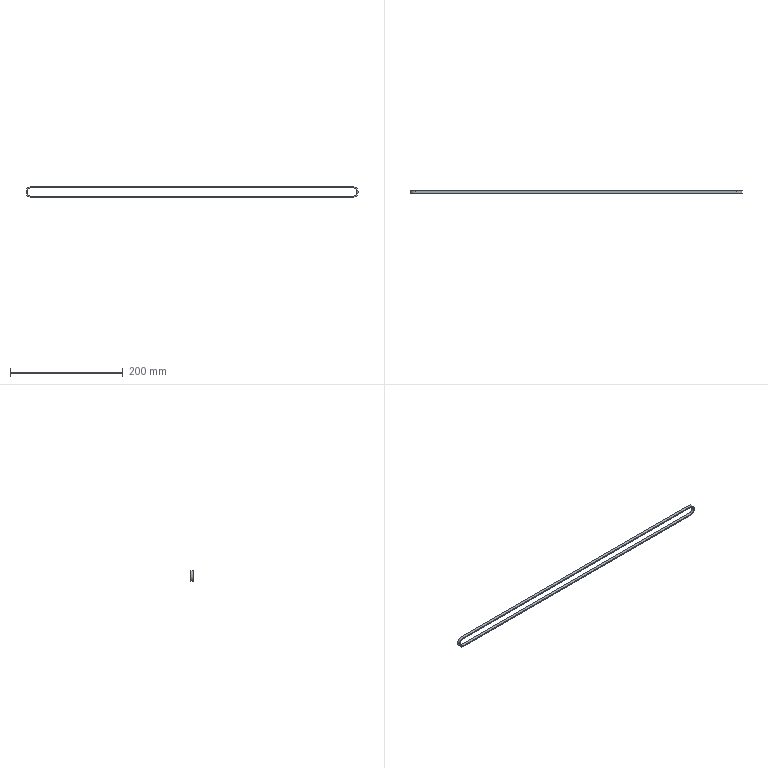Part | SolidWorks | features Extrusion 1 | 1 solid | 10 faces | box 588 x 5 x 19 mm | volume 11914 mm3 | plane 6 | cylinder 4 | commonest cylinder face diameters 15 x2 19 x2
STEP:
#1=CARTESIAN_POINT('',(284.5,5.,9.5));
#2=VERTEX_POINT('',#1);
#3=CARTESIAN_POINT('',(284.5,5.,-9.5));
#4=VERTEX_POINT('',#3);
#5=CARTESIAN_POINT('',(284.5,5.,0.));
#6=DIRECTION('',(0.,1.,0.));
#7=DIRECTION('',(0.,0.,1.));
#8=AXIS2_PLACEMENT_3D('',#5,#6,#7);
#9=CIRCLE('',#8,9.5);
#10=EDGE_CURVE('',#2,#4,#9,.T.);
#11=ORIENTED_EDGE('',*,*,#10,.T.);
#12=CARTESIAN_POINT('',(-284.5,5.,-9.5));
#13=VERTEX_POINT('',#12);
#14=CARTESIAN_POINT('',(284.5,5.,-9.5));
#15=DIRECTION('',(-1.,0.,0.));
#16=VECTOR('',#15,1000.);
#17=LINE('',#14,#16);
#18=EDGE_CURVE('',#4,#13,#17,.T.);
#19=ORIENTED_EDGE('',*,*,#18,.T.);
#20=CARTESIAN_POINT('',(-284.5,5.,9.5));
#21=VERTEX_POINT('',#20);
#22=CARTESIAN_POINT('',(-284.5,5.,0.));
#23=DIRECTION('',(0.,1.,0.));
#24=DIRECTION('',(0.,0.,1.));
#25=AXIS2_PLACEMENT_3D('',#22,#23,#24);
#26=CIRCLE('',#25,9.5);
#27=EDGE_CURVE('',#13,#21,#26,.T.);
#28=ORIENTED_EDGE('',*,*,#27,.T.);
#29=CARTESIAN_POINT('',(284.5,5.,9.5));
#30=DIRECTION('',(1.,0.,0.));
#31=VECTOR('',#30,1000.);
#32=LINE('',#29,#31);
#33=EDGE_CURVE('',#21,#2,#32,.T.);
#34=ORIENTED_EDGE('',*,*,#33,.T.);
#35=EDGE_LOOP('',(#11,#19,#28,#34));
#36=FACE_OUTER_BOUND('',#35,.T.);
#37=CARTESIAN_POINT('',(284.5,5.,-7.5));
#38=VERTEX_POINT('',#37);
#39=CARTESIAN_POINT('',(-284.5,5.,-7.5));
#40=VERTEX_POINT('',#39);
#41=CARTESIAN_POINT('',(284.5,5.,-7.5));
#42=DIRECTION('',(-1.,0.,0.));
#43=VECTOR('',#42,1000.);
#44=LINE('',#41,#43);
#45=EDGE_CURVE('',#38,#40,#44,.T.);
#46=ORIENTED_EDGE('',*,*,#45,.F.);
#47=CARTESIAN_POINT('',(284.5,5.,7.5));
#48=VERTEX_POINT('',#47);
#49=CARTESIAN_POINT('',(284.5,5.,0.));
#50=DIRECTION('',(0.,1.,0.));
#51=DIRECTION('',(0.,0.,1.));
#52=AXIS2_PLACEMENT_3D('',#49,#50,#51);
#53=CIRCLE('',#52,7.5);
#54=EDGE_CURVE('',#48,#38,#53,.T.);
#55=ORIENTED_EDGE('',*,*,#54,.F.);
#56=CARTESIAN_POINT('',(-284.5,5.,7.5));
#57=VERTEX_POINT('',#56);
#58=CARTESIAN_POINT('',(284.5,5.,7.5));
#59=DIRECTION('',(1.,0.,0.));
#60=VECTOR('',#59,1000.);
#61=LINE('',#58,#60);
#62=EDGE_CURVE('',#57,#48,#61,.T.);
#63=ORIENTED_EDGE('',*,*,#62,.F.);
#64=CARTESIAN_POINT('',(-284.5,5.,0.));
#65=DIRECTION('',(0.,1.,0.));
#66=DIRECTION('',(0.,0.,1.));
#67=AXIS2_PLACEMENT_3D('',#64,#65,#66);
#68=CIRCLE('',#67,7.5);
#69=EDGE_CURVE('',#40,#57,#68,.T.);
#70=ORIENTED_EDGE('',*,*,#69,.F.);
#71=EDGE_LOOP('',(#46,#55,#63,#70));
#72=FACE_BOUND('',#71,.T.);
#73=CARTESIAN_POINT('',(284.5,5.,0.));
#74=DIRECTION('',(0.,1.,0.));
#75=DIRECTION('',(0.,0.,1.));
#76=AXIS2_PLACEMENT_3D('',#73,#74,#75);
#77=PLANE('',#76);
#78=ADVANCED_FACE('',(#36,#72),#77,.T.);
#79=CARTESIAN_POINT('',(284.5,0.,9.5));
#80=VERTEX_POINT('',#79);
#81=CARTESIAN_POINT('',(284.5,0.,-9.5));
#82=VERTEX_POINT('',#81);
#83=CARTESIAN_POINT('',(284.5,0.,0.));
#84=DIRECTION('',(0.,1.,0.));
#85=DIRECTION('',(0.,0.,1.));
#86=AXIS2_PLACEMENT_3D('',#83,#84,#85);
#87=CIRCLE('',#86,9.5);
#88=EDGE_CURVE('',#80,#82,#87,.T.);
#89=ORIENTED_EDGE('',*,*,#88,.F.);
#90=CARTESIAN_POINT('',(-284.5,0.,9.5));
#91=VERTEX_POINT('',#90);
#92=CARTESIAN_POINT('',(284.5,0.,9.5));
#93=DIRECTION('',(1.,0.,0.));
#94=VECTOR('',#93,1000.);
#95=LINE('',#92,#94);
#96=EDGE_CURVE('',#91,#80,#95,.T.);
#97=ORIENTED_EDGE('',*,*,#96,.F.);
#98=CARTESIAN_POINT('',(-284.5,0.,-9.5));
#99=VERTEX_POINT('',#98);
#100=CARTESIAN_POINT('',(-284.5,0.,0.));
#101=DIRECTION('',(0.,1.,0.));
#102=DIRECTION('',(0.,0.,1.));
#103=AXIS2_PLACEMENT_3D('',#100,#101,#102);
#104=CIRCLE('',#103,9.5);
#105=EDGE_CURVE('',#99,#91,#104,.T.);
#106=ORIENTED_EDGE('',*,*,#105,.F.);
#107=CARTESIAN_POINT('',(284.5,0.,-9.5));
#108=DIRECTION('',(-1.,0.,0.));
#109=VECTOR('',#108,1000.);
#110=LINE('',#107,#109);
#111=EDGE_CURVE('',#82,#99,#110,.T.);
#112=ORIENTED_EDGE('',*,*,#111,.F.);
#113=EDGE_LOOP('',(#89,#97,#106,#112));
#114=FACE_OUTER_BOUND('',#113,.T.);
#115=CARTESIAN_POINT('',(284.5,0.,7.5));
#116=VERTEX_POINT('',#115);
#117=CARTESIAN_POINT('',(284.5,0.,-7.5));
#118=VERTEX_POINT('',#117);
#119=CARTESIAN_POINT('',(284.5,0.,0.));
#120=DIRECTION('',(0.,1.,0.));
#121=DIRECTION('',(0.,0.,1.));
#122=AXIS2_PLACEMENT_3D('',#119,#120,#121);
#123=CIRCLE('',#122,7.5);
#124=EDGE_CURVE('',#116,#118,#123,.T.);
#125=ORIENTED_EDGE('',*,*,#124,.T.);
#126=CARTESIAN_POINT('',(-284.5,0.,-7.5));
#127=VERTEX_POINT('',#126);
#128=CARTESIAN_POINT('',(284.5,0.,-7.5));
#129=DIRECTION('',(-1.,0.,0.));
#130=VECTOR('',#129,1000.);
#131=LINE('',#128,#130);
#132=EDGE_CURVE('',#118,#127,#131,.T.);
#133=ORIENTED_EDGE('',*,*,#132,.T.);
#134=CARTESIAN_POINT('',(-284.5,0.,7.5));
#135=VERTEX_POINT('',#134);
#136=CARTESIAN_POINT('',(-284.5,0.,0.));
#137=DIRECTION('',(0.,1.,0.));
#138=DIRECTION('',(0.,0.,1.));
#139=AXIS2_PLACEMENT_3D('',#136,#137,#138);
#140=CIRCLE('',#139,7.5);
#141=EDGE_CURVE('',#127,#135,#140,.T.);
#142=ORIENTED_EDGE('',*,*,#141,.T.);
#143=CARTESIAN_POINT('',(284.5,0.,7.5));
#144=DIRECTION('',(1.,0.,0.));
#145=VECTOR('',#144,1000.);
#146=LINE('',#143,#145);
#147=EDGE_CURVE('',#135,#116,#146,.T.);
#148=ORIENTED_EDGE('',*,*,#147,.T.);
#149=EDGE_LOOP('',(#125,#133,#142,#148));
#150=FACE_BOUND('',#149,.T.);
#151=CARTESIAN_POINT('',(284.5,0.,0.));
#152=DIRECTION('',(0.,1.,0.));
#153=DIRECTION('',(0.,0.,1.));
#154=AXIS2_PLACEMENT_3D('',#151,#152,#153);
#155=PLANE('',#154);
#156=ADVANCED_FACE('',(#114,#150),#155,.F.);
#157=ORIENTED_EDGE('',*,*,#88,.T.);
#158=CARTESIAN_POINT('',(284.5,5.,-9.5));
#159=DIRECTION('',(0.,-1.,0.));
#160=VECTOR('',#159,1000.);
#161=LINE('',#158,#160);
#162=EDGE_CURVE('',#4,#82,#161,.T.);
#163=ORIENTED_EDGE('',*,*,#162,.F.);
#164=ORIENTED_EDGE('',*,*,#10,.F.);
#165=CARTESIAN_POINT('',(284.5,5.,9.5));
#166=DIRECTION('',(0.,-1.,0.));
#167=VECTOR('',#166,1000.);
#168=LINE('',#165,#167);
#169=EDGE_CURVE('',#2,#80,#168,.T.);
#170=ORIENTED_EDGE('',*,*,#169,.T.);
#171=EDGE_LOOP('',(#157,#163,#164,#170));
#172=FACE_OUTER_BOUND('',#171,.T.);
#173=CARTESIAN_POINT('',(284.5,5.,0.));
#174=DIRECTION('',(0.,-1.,0.));
#175=DIRECTION('',(0.,0.,-1.));
#176=AXIS2_PLACEMENT_3D('',#173,#174,#175);
#177=CYLINDRICAL_SURFACE('',#176,9.5);
#178=ADVANCED_FACE('',(#172),#177,.T.);
#179=ORIENTED_EDGE('',*,*,#111,.T.);
#180=CARTESIAN_POINT('',(-284.5,5.,-9.5));
#181=DIRECTION('',(0.,-1.,0.));
#182=VECTOR('',#181,1000.);
#183=LINE('',#180,#182);
#184=EDGE_CURVE('',#13,#99,#183,.T.);
#185=ORIENTED_EDGE('',*,*,#184,.F.);
#186=ORIENTED_EDGE('',*,*,#18,.F.);
#187=ORIENTED_EDGE('',*,*,#162,.T.);
#188=EDGE_LOOP('',(#179,#185,#186,#187));
#189=FACE_OUTER_BOUND('',#188,.T.);
#190=CARTESIAN_POINT('',(284.5,5.,-9.5));
#191=DIRECTION('',(0.,0.,1.));
#192=DIRECTION('',(1.,0.,0.));
#193=AXIS2_PLACEMENT_3D('',#190,#191,#192);
#194=PLANE('',#193);
#195=ADVANCED_FACE('',(#189),#194,.F.);
#196=ORIENTED_EDGE('',*,*,#105,.T.);
#197=CARTESIAN_POINT('',(-284.5,5.,9.5));
#198=DIRECTION('',(0.,-1.,0.));
#199=VECTOR('',#198,1000.);
#200=LINE('',#197,#199);
#201=EDGE_CURVE('',#21,#91,#200,.T.);
#202=ORIENTED_EDGE('',*,*,#201,.F.);
#203=ORIENTED_EDGE('',*,*,#27,.F.);
#204=ORIENTED_EDGE('',*,*,#184,.T.);
#205=EDGE_LOOP('',(#196,#202,#203,#204));
#206=FACE_OUTER_BOUND('',#205,.T.);
#207=CARTESIAN_POINT('',(-284.5,5.,0.));
#208=DIRECTION('',(0.,-1.,0.));
#209=DIRECTION('',(0.,0.,-1.));
#210=AXIS2_PLACEMENT_3D('',#207,#208,#209);
#211=CYLINDRICAL_SURFACE('',#210,9.5);
#212=ADVANCED_FACE('',(#206),#211,.T.);
#213=ORIENTED_EDGE('',*,*,#96,.T.);
#214=ORIENTED_EDGE('',*,*,#169,.F.);
#215=ORIENTED_EDGE('',*,*,#33,.F.);
#216=ORIENTED_EDGE('',*,*,#201,.T.);
#217=EDGE_LOOP('',(#213,#214,#215,#216));
#218=FACE_OUTER_BOUND('',#217,.T.);
#219=CARTESIAN_POINT('',(284.5,5.,9.5));
#220=DIRECTION('',(0.,0.,-1.));
#221=DIRECTION('',(-1.,0.,0.));
#222=AXIS2_PLACEMENT_3D('',#219,#220,#221);
#223=PLANE('',#222);
#224=ADVANCED_FACE('',(#218),#223,.F.);
#225=ORIENTED_EDGE('',*,*,#124,.F.);
#226=CARTESIAN_POINT('',(284.5,5.,7.5));
#227=DIRECTION('',(0.,-1.,0.));
#228=VECTOR('',#227,1000.);
#229=LINE('',#226,#228);
#230=EDGE_CURVE('',#48,#116,#229,.T.);
#231=ORIENTED_EDGE('',*,*,#230,.F.);
#232=ORIENTED_EDGE('',*,*,#54,.T.);
#233=CARTESIAN_POINT('',(284.5,5.,-7.5));
#234=DIRECTION('',(0.,-1.,0.));
#235=VECTOR('',#234,1000.);
#236=LINE('',#233,#235);
#237=EDGE_CURVE('',#38,#118,#236,.T.);
#238=ORIENTED_EDGE('',*,*,#237,.T.);
#239=EDGE_LOOP('',(#225,#231,#232,#238));
#240=FACE_OUTER_BOUND('',#239,.T.);
#241=CARTESIAN_POINT('',(284.5,5.,0.));
#242=DIRECTION('',(0.,-1.,0.));
#243=DIRECTION('',(0.,0.,-1.));
#244=AXIS2_PLACEMENT_3D('',#241,#242,#243);
#245=CYLINDRICAL_SURFACE('',#244,7.5);
#246=ADVANCED_FACE('',(#240),#245,.F.);
#247=ORIENTED_EDGE('',*,*,#132,.F.);
#248=ORIENTED_EDGE('',*,*,#237,.F.);
#249=ORIENTED_EDGE('',*,*,#45,.T.);
#250=CARTESIAN_POINT('',(-284.5,5.,-7.5));
#251=DIRECTION('',(0.,-1.,0.));
#252=VECTOR('',#251,1000.);
#253=LINE('',#250,#252);
#254=EDGE_CURVE('',#40,#127,#253,.T.);
#255=ORIENTED_EDGE('',*,*,#254,.T.);
#256=EDGE_LOOP('',(#247,#248,#249,#255));
#257=FACE_OUTER_BOUND('',#256,.T.);
#258=CARTESIAN_POINT('',(284.5,5.,-7.5));
#259=DIRECTION('',(0.,0.,1.));
#260=DIRECTION('',(1.,0.,0.));
#261=AXIS2_PLACEMENT_3D('',#258,#259,#260);
#262=PLANE('',#261);
#263=ADVANCED_FACE('',(#257),#262,.T.);
#264=ORIENTED_EDGE('',*,*,#141,.F.);
#265=ORIENTED_EDGE('',*,*,#254,.F.);
#266=ORIENTED_EDGE('',*,*,#69,.T.);
#267=CARTESIAN_POINT('',(-284.5,5.,7.5));
#268=DIRECTION('',(0.,-1.,0.));
#269=VECTOR('',#268,1000.);
#270=LINE('',#267,#269);
#271=EDGE_CURVE('',#57,#135,#270,.T.);
#272=ORIENTED_EDGE('',*,*,#271,.T.);
#273=EDGE_LOOP('',(#264,#265,#266,#272));
#274=FACE_OUTER_BOUND('',#273,.T.);
#275=CARTESIAN_POINT('',(-284.5,5.,0.));
#276=DIRECTION('',(0.,-1.,0.));
#277=DIRECTION('',(0.,0.,-1.));
#278=AXIS2_PLACEMENT_3D('',#275,#276,#277);
#279=CYLINDRICAL_SURFACE('',#278,7.5);
#280=ADVANCED_FACE('',(#274),#279,.F.);
#281=ORIENTED_EDGE('',*,*,#147,.F.);
#282=ORIENTED_EDGE('',*,*,#271,.F.);
#283=ORIENTED_EDGE('',*,*,#62,.T.);
#284=ORIENTED_EDGE('',*,*,#230,.T.);
#285=EDGE_LOOP('',(#281,#282,#283,#284));
#286=FACE_OUTER_BOUND('',#285,.T.);
#287=CARTESIAN_POINT('',(284.5,5.,7.5));
#288=DIRECTION('',(0.,0.,-1.));
#289=DIRECTION('',(-1.,0.,0.));
#290=AXIS2_PLACEMENT_3D('',#287,#288,#289);
#291=PLANE('',#290);
#292=ADVANCED_FACE('',(#286),#291,.T.);
#293=CLOSED_SHELL('',(#78,#156,#178,#195,#212,#224,#246,#263,#280,#292));
#294=MANIFOLD_SOLID_BREP('',#293);
#295=CARTESIAN_POINT('',(0.,0.,0.));
#296=DIRECTION('',(0.,0.,1.));
#297=DIRECTION('',(1.,0.,0.));
#298=AXIS2_PLACEMENT_3D('',#295,#296,#297);
#299=(LENGTH_UNIT()NAMED_UNIT(*)SI_UNIT(.MILLI.,.METRE.));
#300=UNCERTAINTY_MEASURE_WITH_UNIT(LENGTH_MEASURE(0.00001),#299,'','');
#301=(NAMED_UNIT(*)PLANE_ANGLE_UNIT()SI_UNIT($,.RADIAN.));
#302=(NAMED_UNIT(*)SI_UNIT($,.STERADIAN.)SOLID_ANGLE_UNIT());
#303=(GEOMETRIC_REPRESENTATION_CONTEXT(3)GLOBAL_UNCERTAINTY_ASSIGNED_CONTEXT((#300))GLOBAL_UNIT_ASSIGNED_CONTEXT((#299,#301,#302))REPRESENTATION_CONTEXT('',''));
#304=ADVANCED_BREP_SHAPE_REPRESENTATION('',(#294,#298),#303);